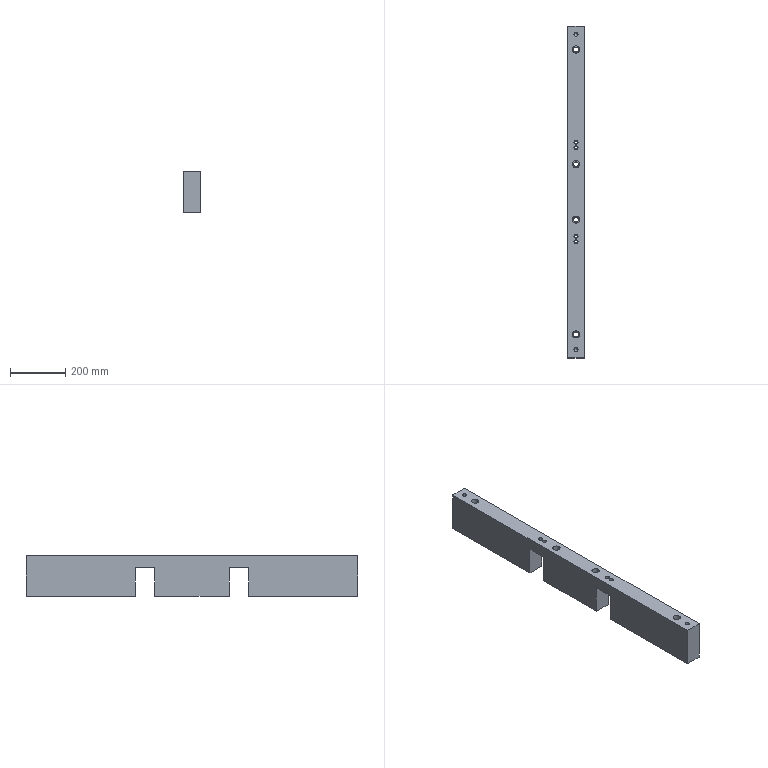Part | STEP file | lll_id2306_x_t | 1 solid | 42 faces | box 60 x 1200 x 147.5 mm | volume 9489564 mm3 | plane 22 | cylinder 18 | cone 2 | commonest cylinder face diameters 9.009 x4 14.508 x4 18.009 x4 26.008 x4 14.506 x2
STEP:
#1=CARTESIAN_POINT('',(1904.254,-179.998,370.));
#2=VERTEX_POINT('',#1);
#3=CARTESIAN_POINT('',(1897.,-179.998,370.));
#4=DIRECTION('',(0.,0.,-1.));
#5=DIRECTION('',(1.,0.,0.));
#6=AXIS2_PLACEMENT_3D('',#3,#4,#5);
#7=CIRCLE('',#6,7.254);
#8=EDGE_CURVE('',#2,#2,#7,.T.);
#9=ORIENTED_EDGE('',*,*,#8,.T.);
#10=EDGE_LOOP('',(#9));
#11=FACE_BOUND('',#10,.T.);
#12=CARTESIAN_POINT('',(1904.254,-159.998,370.));
#13=VERTEX_POINT('',#12);
#14=CARTESIAN_POINT('',(1897.,-159.998,370.));
#15=DIRECTION('',(0.,0.,-1.));
#16=DIRECTION('',(1.,0.,0.));
#17=AXIS2_PLACEMENT_3D('',#14,#15,#16);
#18=CIRCLE('',#17,7.254);
#19=EDGE_CURVE('',#13,#13,#18,.T.);
#20=ORIENTED_EDGE('',*,*,#19,.T.);
#21=EDGE_LOOP('',(#20));
#22=FACE_BOUND('',#21,.T.);
#23=CARTESIAN_POINT('',(1904.254,160.,370.));
#24=VERTEX_POINT('',#23);
#25=CARTESIAN_POINT('',(1897.,160.,370.));
#26=DIRECTION('',(0.,0.,-1.));
#27=DIRECTION('',(1.,0.,0.));
#28=AXIS2_PLACEMENT_3D('',#25,#26,#27);
#29=CIRCLE('',#28,7.254);
#30=EDGE_CURVE('',#24,#24,#29,.T.);
#31=ORIENTED_EDGE('',*,*,#30,.T.);
#32=EDGE_LOOP('',(#31));
#33=FACE_BOUND('',#32,.T.);
#34=CARTESIAN_POINT('',(1904.254,180.,370.));
#35=VERTEX_POINT('',#34);
#36=CARTESIAN_POINT('',(1897.,180.,370.));
#37=DIRECTION('',(0.,0.,-1.));
#38=DIRECTION('',(1.,0.,0.));
#39=AXIS2_PLACEMENT_3D('',#36,#37,#38);
#40=CIRCLE('',#39,7.254);
#41=EDGE_CURVE('',#35,#35,#40,.T.);
#42=ORIENTED_EDGE('',*,*,#41,.T.);
#43=EDGE_LOOP('',(#42));
#44=FACE_BOUND('',#43,.T.);
#45=CARTESIAN_POINT('',(1910.004,100.,370.));
#46=VERTEX_POINT('',#45);
#47=CARTESIAN_POINT('',(1897.,100.,370.));
#48=DIRECTION('',(0.,0.,1.));
#49=DIRECTION('',(1.,0.,0.));
#50=AXIS2_PLACEMENT_3D('',#47,#48,#49);
#51=CIRCLE('',#50,13.004);
#52=EDGE_CURVE('',#46,#46,#51,.T.);
#53=ORIENTED_EDGE('',*,*,#52,.F.);
#54=EDGE_LOOP('',(#53));
#55=FACE_BOUND('',#54,.T.);
#56=CARTESIAN_POINT('',(1910.004,-100.,370.));
#57=VERTEX_POINT('',#56);
#58=CARTESIAN_POINT('',(1897.,-100.,370.));
#59=DIRECTION('',(0.,0.,-1.));
#60=DIRECTION('',(1.,0.,0.));
#61=AXIS2_PLACEMENT_3D('',#58,#59,#60);
#62=CIRCLE('',#61,13.004);
#63=EDGE_CURVE('',#57,#57,#62,.T.);
#64=ORIENTED_EDGE('',*,*,#63,.T.);
#65=EDGE_LOOP('',(#64));
#66=FACE_BOUND('',#65,.T.);
#67=CARTESIAN_POINT('',(1910.004,-515.,370.));
#68=VERTEX_POINT('',#67);
#69=CARTESIAN_POINT('',(1897.,-515.,370.));
#70=DIRECTION('',(0.,0.,-1.));
#71=DIRECTION('',(1.,0.,0.));
#72=AXIS2_PLACEMENT_3D('',#69,#70,#71);
#73=CIRCLE('',#72,13.004);
#74=EDGE_CURVE('',#68,#68,#73,.T.);
#75=ORIENTED_EDGE('',*,*,#74,.T.);
#76=EDGE_LOOP('',(#75));
#77=FACE_BOUND('',#76,.T.);
#78=CARTESIAN_POINT('',(1927.,600.,370.));
#79=VERTEX_POINT('',#78);
#80=CARTESIAN_POINT('',(1867.,600.,370.));
#81=VERTEX_POINT('',#80);
#82=CARTESIAN_POINT('',(5837.,600.,370.));
#83=DIRECTION('',(-1.,0.,0.));
#84=VECTOR('',#83,1.);
#85=LINE('',#82,#84);
#86=EDGE_CURVE('',#79,#81,#85,.T.);
#87=ORIENTED_EDGE('',*,*,#86,.T.);
#88=CARTESIAN_POINT('',(1867.,-600.,370.));
#89=VERTEX_POINT('',#88);
#90=CARTESIAN_POINT('',(1867.,600.,370.));
#91=DIRECTION('',(0.,-1.,0.));
#92=VECTOR('',#91,1.);
#93=LINE('',#90,#92);
#94=EDGE_CURVE('',#81,#89,#93,.T.);
#95=ORIENTED_EDGE('',*,*,#94,.T.);
#96=CARTESIAN_POINT('',(1927.,-600.,370.));
#97=VERTEX_POINT('',#96);
#98=CARTESIAN_POINT('',(1867.,-600.,370.));
#99=DIRECTION('',(1.,0.,0.));
#100=VECTOR('',#99,1.);
#101=LINE('',#98,#100);
#102=EDGE_CURVE('',#89,#97,#101,.T.);
#103=ORIENTED_EDGE('',*,*,#102,.T.);
#104=CARTESIAN_POINT('',(1927.,1.,370.));
#105=DIRECTION('',(0.,1.,0.));
#106=VECTOR('',#105,1.);
#107=LINE('',#104,#106);
#108=EDGE_CURVE('',#97,#79,#107,.T.);
#109=ORIENTED_EDGE('',*,*,#108,.T.);
#110=EDGE_LOOP('',(#87,#95,#103,#109));
#111=FACE_BOUND('',#110,.T.);
#112=CARTESIAN_POINT('',(1910.004,515.,370.));
#113=VERTEX_POINT('',#112);
#114=CARTESIAN_POINT('',(1897.,515.,370.));
#115=DIRECTION('',(0.,0.,1.));
#116=DIRECTION('',(1.,0.,0.));
#117=AXIS2_PLACEMENT_3D('',#114,#115,#116);
#118=CIRCLE('',#117,13.004);
#119=EDGE_CURVE('',#113,#113,#118,.T.);
#120=ORIENTED_EDGE('',*,*,#119,.F.);
#121=EDGE_LOOP('',(#120));
#122=FACE_BOUND('',#121,.T.);
#123=CARTESIAN_POINT('',(1904.253,-570.,370.));
#124=VERTEX_POINT('',#123);
#125=CARTESIAN_POINT('',(1897.,-570.,370.));
#126=DIRECTION('',(0.,0.,-1.));
#127=DIRECTION('',(1.,0.,0.));
#128=AXIS2_PLACEMENT_3D('',#125,#126,#127);
#129=CIRCLE('',#128,7.253);
#130=EDGE_CURVE('',#124,#124,#129,.T.);
#131=ORIENTED_EDGE('',*,*,#130,.T.);
#132=EDGE_LOOP('',(#131));
#133=FACE_BOUND('',#132,.T.);
#134=CARTESIAN_POINT('',(1904.253,570.,370.));
#135=VERTEX_POINT('',#134);
#136=CARTESIAN_POINT('',(1897.,570.,370.));
#137=DIRECTION('',(0.,0.,1.));
#138=DIRECTION('',(1.,0.,0.));
#139=AXIS2_PLACEMENT_3D('',#136,#137,#138);
#140=CIRCLE('',#139,7.253);
#141=EDGE_CURVE('',#135,#135,#140,.T.);
#142=ORIENTED_EDGE('',*,*,#141,.F.);
#143=EDGE_LOOP('',(#142));
#144=FACE_BOUND('',#143,.T.);
#145=CARTESIAN_POINT('',(-319.315,1.,370.));
#146=DIRECTION('',(0.,0.,-1.));
#147=DIRECTION('',(1.,0.,0.));
#148=AXIS2_PLACEMENT_3D('',#145,#146,#147);
#149=PLANE('',#148);
#150=ADVANCED_FACE('',(#11,#22,#33,#44,#55,#66,#77,#111,#122,#133,#144),#149,.F.);
#151=CARTESIAN_POINT('',(1887.995,-100.,222.5));
#152=VERTEX_POINT('',#151);
#153=CARTESIAN_POINT('',(1897.,-100.,222.5));
#154=DIRECTION('',(0.,0.,1.));
#155=DIRECTION('',(-1.,0.,0.));
#156=AXIS2_PLACEMENT_3D('',#153,#154,#155);
#157=CIRCLE('',#156,9.005);
#158=EDGE_CURVE('',#152,#152,#157,.T.);
#159=ORIENTED_EDGE('',*,*,#158,.T.);
#160=EDGE_LOOP('',(#159));
#161=FACE_BOUND('',#160,.T.);
#162=CARTESIAN_POINT('',(1887.995,100.,222.5));
#163=VERTEX_POINT('',#162);
#164=CARTESIAN_POINT('',(1897.,100.,222.5));
#165=DIRECTION('',(0.,0.,-1.));
#166=DIRECTION('',(-1.,0.,0.));
#167=AXIS2_PLACEMENT_3D('',#164,#165,#166);
#168=CIRCLE('',#167,9.005);
#169=EDGE_CURVE('',#163,#163,#168,.T.);
#170=ORIENTED_EDGE('',*,*,#169,.F.);
#171=EDGE_LOOP('',(#170));
#172=FACE_BOUND('',#171,.T.);
#173=CARTESIAN_POINT('',(1927.,135.249,222.5));
#174=VERTEX_POINT('',#173);
#175=CARTESIAN_POINT('',(1867.,135.249,222.5));
#176=VERTEX_POINT('',#175);
#177=CARTESIAN_POINT('',(-319.315,135.249,222.5));
#178=DIRECTION('',(-1.,0.,0.));
#179=VECTOR('',#178,1.);
#180=LINE('',#177,#179);
#181=EDGE_CURVE('',#174,#176,#180,.T.);
#182=ORIENTED_EDGE('',*,*,#181,.F.);
#183=CARTESIAN_POINT('',(1927.,-134.749,222.5));
#184=VERTEX_POINT('',#183);
#185=CARTESIAN_POINT('',(1927.,1.,222.5));
#186=DIRECTION('',(0.,-1.,0.));
#187=VECTOR('',#186,1.);
#188=LINE('',#185,#187);
#189=EDGE_CURVE('',#174,#184,#188,.T.);
#190=ORIENTED_EDGE('',*,*,#189,.T.);
#191=CARTESIAN_POINT('',(1867.,-134.749,222.5));
#192=VERTEX_POINT('',#191);
#193=CARTESIAN_POINT('',(-319.315,-134.749,222.5));
#194=DIRECTION('',(1.,0.,0.));
#195=VECTOR('',#194,1.);
#196=LINE('',#193,#195);
#197=EDGE_CURVE('',#192,#184,#196,.T.);
#198=ORIENTED_EDGE('',*,*,#197,.F.);
#199=CARTESIAN_POINT('',(1867.,600.,222.5));
#200=DIRECTION('',(0.,-1.,0.));
#201=VECTOR('',#200,1.);
#202=LINE('',#199,#201);
#203=EDGE_CURVE('',#176,#192,#202,.T.);
#204=ORIENTED_EDGE('',*,*,#203,.F.);
#205=EDGE_LOOP('',(#182,#190,#198,#204));
#206=FACE_BOUND('',#205,.T.);
#207=CARTESIAN_POINT('',(-319.315,1.,222.5));
#208=DIRECTION('',(0.,0.,-1.));
#209=DIRECTION('',(1.,0.,0.));
#210=AXIS2_PLACEMENT_3D('',#207,#208,#209);
#211=PLANE('',#210);
#212=ADVANCED_FACE('',(#161,#172,#206),#211,.T.);
#213=CARTESIAN_POINT('',(1867.,205.249,222.5));
#214=VERTEX_POINT('',#213);
#215=CARTESIAN_POINT('',(1927.,205.249,222.5));
#216=VERTEX_POINT('',#215);
#217=CARTESIAN_POINT('',(-319.315,205.249,222.5));
#218=DIRECTION('',(1.,0.,0.));
#219=VECTOR('',#218,1.);
#220=LINE('',#217,#219);
#221=EDGE_CURVE('',#214,#216,#220,.T.);
#222=ORIENTED_EDGE('',*,*,#221,.F.);
#223=CARTESIAN_POINT('',(1867.,600.,222.5));
#224=VERTEX_POINT('',#223);
#225=CARTESIAN_POINT('',(1867.,600.,222.5));
#226=DIRECTION('',(0.,-1.,0.));
#227=VECTOR('',#226,1.);
#228=LINE('',#225,#227);
#229=EDGE_CURVE('',#224,#214,#228,.T.);
#230=ORIENTED_EDGE('',*,*,#229,.F.);
#231=CARTESIAN_POINT('',(1927.,600.,222.5));
#232=VERTEX_POINT('',#231);
#233=CARTESIAN_POINT('',(5837.,600.,222.5));
#234=DIRECTION('',(-1.,0.,0.));
#235=VECTOR('',#234,1.);
#236=LINE('',#233,#235);
#237=EDGE_CURVE('',#232,#224,#236,.T.);
#238=ORIENTED_EDGE('',*,*,#237,.F.);
#239=CARTESIAN_POINT('',(1927.,1.,222.5));
#240=DIRECTION('',(0.,-1.,0.));
#241=VECTOR('',#240,1.);
#242=LINE('',#239,#241);
#243=EDGE_CURVE('',#232,#216,#242,.T.);
#244=ORIENTED_EDGE('',*,*,#243,.T.);
#245=EDGE_LOOP('',(#222,#230,#238,#244));
#246=FACE_BOUND('',#245,.T.);
#247=CARTESIAN_POINT('',(1906.005,515.,222.5));
#248=VERTEX_POINT('',#247);
#249=CARTESIAN_POINT('',(1897.,515.,222.5));
#250=DIRECTION('',(0.,0.,-1.));
#251=DIRECTION('',(1.,0.,0.));
#252=AXIS2_PLACEMENT_3D('',#249,#250,#251);
#253=CIRCLE('',#252,9.005);
#254=EDGE_CURVE('',#248,#248,#253,.T.);
#255=ORIENTED_EDGE('',*,*,#254,.F.);
#256=EDGE_LOOP('',(#255));
#257=FACE_BOUND('',#256,.T.);
#258=CARTESIAN_POINT('',(-319.315,1.,222.5));
#259=DIRECTION('',(0.,0.,-1.));
#260=DIRECTION('',(1.,0.,0.));
#261=AXIS2_PLACEMENT_3D('',#258,#259,#260);
#262=PLANE('',#261);
#263=ADVANCED_FACE('',(#246,#257),#262,.T.);
#264=CARTESIAN_POINT('',(1927.,-204.749,222.5));
#265=VERTEX_POINT('',#264);
#266=CARTESIAN_POINT('',(1867.,-204.749,222.5));
#267=VERTEX_POINT('',#266);
#268=CARTESIAN_POINT('',(-319.315,-204.749,222.5));
#269=DIRECTION('',(-1.,0.,0.));
#270=VECTOR('',#269,1.);
#271=LINE('',#268,#270);
#272=EDGE_CURVE('',#265,#267,#271,.T.);
#273=ORIENTED_EDGE('',*,*,#272,.F.);
#274=CARTESIAN_POINT('',(1927.,-600.,222.5));
#275=VERTEX_POINT('',#274);
#276=CARTESIAN_POINT('',(1927.,1.,222.5));
#277=DIRECTION('',(0.,-1.,0.));
#278=VECTOR('',#277,1.);
#279=LINE('',#276,#278);
#280=EDGE_CURVE('',#265,#275,#279,.T.);
#281=ORIENTED_EDGE('',*,*,#280,.T.);
#282=CARTESIAN_POINT('',(1867.,-600.,222.5));
#283=VERTEX_POINT('',#282);
#284=CARTESIAN_POINT('',(1867.,-600.,222.5));
#285=DIRECTION('',(1.,0.,0.));
#286=VECTOR('',#285,1.);
#287=LINE('',#284,#286);
#288=EDGE_CURVE('',#283,#275,#287,.T.);
#289=ORIENTED_EDGE('',*,*,#288,.F.);
#290=CARTESIAN_POINT('',(1867.,600.,222.5));
#291=DIRECTION('',(0.,-1.,0.));
#292=VECTOR('',#291,1.);
#293=LINE('',#290,#292);
#294=EDGE_CURVE('',#267,#283,#293,.T.);
#295=ORIENTED_EDGE('',*,*,#294,.F.);
#296=EDGE_LOOP('',(#273,#281,#289,#295));
#297=FACE_BOUND('',#296,.T.);
#298=CARTESIAN_POINT('',(1906.005,-515.,222.5));
#299=VERTEX_POINT('',#298);
#300=CARTESIAN_POINT('',(1897.,-515.,222.5));
#301=DIRECTION('',(0.,0.,1.));
#302=DIRECTION('',(1.,0.,0.));
#303=AXIS2_PLACEMENT_3D('',#300,#301,#302);
#304=CIRCLE('',#303,9.005);
#305=EDGE_CURVE('',#299,#299,#304,.T.);
#306=ORIENTED_EDGE('',*,*,#305,.T.);
#307=EDGE_LOOP('',(#306));
#308=FACE_BOUND('',#307,.T.);
#309=CARTESIAN_POINT('',(-319.315,1.,222.5));
#310=DIRECTION('',(0.,0.,-1.));
#311=DIRECTION('',(1.,0.,0.));
#312=AXIS2_PLACEMENT_3D('',#309,#310,#311);
#313=PLANE('',#312);
#314=ADVANCED_FACE('',(#297,#308),#313,.T.);
#315=CARTESIAN_POINT('',(1867.,-134.749,326.5));
#316=VERTEX_POINT('',#315);
#317=CARTESIAN_POINT('',(1867.,-204.749,326.5));
#318=VERTEX_POINT('',#317);
#319=CARTESIAN_POINT('',(1867.,80.002,326.5));
#320=DIRECTION('',(0.,-1.,0.));
#321=VECTOR('',#320,1.);
#322=LINE('',#319,#321);
#323=EDGE_CURVE('',#316,#318,#322,.T.);
#324=ORIENTED_EDGE('',*,*,#323,.T.);
#325=CARTESIAN_POINT('',(1867.,-204.749,363.5));
#326=DIRECTION('',(0.,0.,1.));
#327=VECTOR('',#326,1.);
#328=LINE('',#325,#327);
#329=EDGE_CURVE('',#267,#318,#328,.T.);
#330=ORIENTED_EDGE('',*,*,#329,.F.);
#331=ORIENTED_EDGE('',*,*,#294,.T.);
#332=CARTESIAN_POINT('',(1867.,-600.,310.));
#333=DIRECTION('',(0.,0.,-1.));
#334=VECTOR('',#333,1.);
#335=LINE('',#332,#334);
#336=EDGE_CURVE('',#89,#283,#335,.T.);
#337=ORIENTED_EDGE('',*,*,#336,.F.);
#338=ORIENTED_EDGE('',*,*,#94,.F.);
#339=CARTESIAN_POINT('',(1867.,600.,310.));
#340=DIRECTION('',(0.,0.,-1.));
#341=VECTOR('',#340,1.);
#342=LINE('',#339,#341);
#343=EDGE_CURVE('',#81,#224,#342,.T.);
#344=ORIENTED_EDGE('',*,*,#343,.T.);
#345=ORIENTED_EDGE('',*,*,#229,.T.);
#346=CARTESIAN_POINT('',(1867.,205.249,326.5));
#347=VERTEX_POINT('',#346);
#348=CARTESIAN_POINT('',(1867.,205.249,363.5));
#349=DIRECTION('',(0.,0.,-1.));
#350=VECTOR('',#349,1.);
#351=LINE('',#348,#350);
#352=EDGE_CURVE('',#347,#214,#351,.T.);
#353=ORIENTED_EDGE('',*,*,#352,.F.);
#354=CARTESIAN_POINT('',(1867.,135.249,326.5));
#355=VERTEX_POINT('',#354);
#356=CARTESIAN_POINT('',(1867.,420.,326.5));
#357=DIRECTION('',(0.,-1.,0.));
#358=VECTOR('',#357,1.);
#359=LINE('',#356,#358);
#360=EDGE_CURVE('',#347,#355,#359,.T.);
#361=ORIENTED_EDGE('',*,*,#360,.T.);
#362=CARTESIAN_POINT('',(1867.,135.249,363.5));
#363=DIRECTION('',(0.,0.,1.));
#364=VECTOR('',#363,1.);
#365=LINE('',#362,#364);
#366=EDGE_CURVE('',#176,#355,#365,.T.);
#367=ORIENTED_EDGE('',*,*,#366,.F.);
#368=ORIENTED_EDGE('',*,*,#203,.T.);
#369=CARTESIAN_POINT('',(1867.,-134.749,363.5));
#370=DIRECTION('',(0.,0.,-1.));
#371=VECTOR('',#370,1.);
#372=LINE('',#369,#371);
#373=EDGE_CURVE('',#316,#192,#372,.T.);
#374=ORIENTED_EDGE('',*,*,#373,.F.);
#375=EDGE_LOOP('',(#324,#330,#331,#337,#338,#344,#345,#353,#361,#367,#368,#374));
#376=FACE_OUTER_BOUND('',#375,.T.);
#377=CARTESIAN_POINT('',(1867.,600.,310.));
#378=DIRECTION('',(-1.,0.,0.));
#379=DIRECTION('',(0.,0.,-1.));
#380=AXIS2_PLACEMENT_3D('',#377,#378,#379);
#381=PLANE('',#380);
#382=ADVANCED_FACE('',(#376),#381,.T.);
#383=CARTESIAN_POINT('',(1927.,-600.,310.));
#384=DIRECTION('',(0.,0.,-1.));
#385=VECTOR('',#384,1.);
#386=LINE('',#383,#385);
#387=EDGE_CURVE('',#97,#275,#386,.T.);
#388=ORIENTED_EDGE('',*,*,#387,.F.);
#389=ORIENTED_EDGE('',*,*,#102,.F.);
#390=ORIENTED_EDGE('',*,*,#336,.T.);
#391=ORIENTED_EDGE('',*,*,#288,.T.);
#392=EDGE_LOOP('',(#388,#389,#390,#391));
#393=FACE_OUTER_BOUND('',#392,.T.);
#394=CARTESIAN_POINT('',(1867.,-600.,310.));
#395=DIRECTION('',(0.,-1.,0.));
#396=DIRECTION('',(0.,0.,-1.));
#397=AXIS2_PLACEMENT_3D('',#394,#395,#396);
#398=PLANE('',#397);
#399=ADVANCED_FACE('',(#393),#398,.T.);
#400=CARTESIAN_POINT('',(1927.,600.,310.));
#401=DIRECTION('',(0.,0.,1.));
#402=VECTOR('',#401,1.);
#403=LINE('',#400,#402);
#404=EDGE_CURVE('',#232,#79,#403,.T.);
#405=ORIENTED_EDGE('',*,*,#404,.F.);
#406=ORIENTED_EDGE('',*,*,#237,.T.);
#407=ORIENTED_EDGE('',*,*,#343,.F.);
#408=ORIENTED_EDGE('',*,*,#86,.F.);
#409=EDGE_LOOP('',(#405,#406,#407,#408));
#410=FACE_OUTER_BOUND('',#409,.T.);
#411=CARTESIAN_POINT('',(5837.,600.,310.));
#412=DIRECTION('',(0.,1.,0.));
#413=DIRECTION('',(0.,0.,1.));
#414=AXIS2_PLACEMENT_3D('',#411,#412,#413);
#415=PLANE('',#414);
#416=ADVANCED_FACE('',(#410),#415,.T.);
#417=CARTESIAN_POINT('',(1927.,-204.749,326.5));
#418=VERTEX_POINT('',#417);
#419=CARTESIAN_POINT('',(1927.,-204.749,294.75));
#420=DIRECTION('',(0.,0.,1.));
#421=VECTOR('',#420,1.);
#422=LINE('',#419,#421);
#423=EDGE_CURVE('',#265,#418,#422,.T.);
#424=ORIENTED_EDGE('',*,*,#423,.T.);
#425=CARTESIAN_POINT('',(1927.,-134.749,326.5));
#426=VERTEX_POINT('',#425);
#427=CARTESIAN_POINT('',(1927.,-519.998,326.5));
#428=DIRECTION('',(0.,-1.,0.));
#429=VECTOR('',#428,1.);
#430=LINE('',#427,#429);
#431=EDGE_CURVE('',#426,#418,#430,.T.);
#432=ORIENTED_EDGE('',*,*,#431,.F.);
#433=CARTESIAN_POINT('',(1927.,-134.749,294.75));
#434=DIRECTION('',(0.,0.,-1.));
#435=VECTOR('',#434,1.);
#436=LINE('',#433,#435);
#437=EDGE_CURVE('',#426,#184,#436,.T.);
#438=ORIENTED_EDGE('',*,*,#437,.T.);
#439=ORIENTED_EDGE('',*,*,#189,.F.);
#440=CARTESIAN_POINT('',(1927.,135.249,326.5));
#441=VERTEX_POINT('',#440);
#442=CARTESIAN_POINT('',(1927.,135.249,294.75));
#443=DIRECTION('',(0.,0.,1.));
#444=VECTOR('',#443,1.);
#445=LINE('',#442,#444);
#446=EDGE_CURVE('',#174,#441,#445,.T.);
#447=ORIENTED_EDGE('',*,*,#446,.T.);
#448=CARTESIAN_POINT('',(1927.,205.249,326.5));
#449=VERTEX_POINT('',#448);
#450=CARTESIAN_POINT('',(1927.,-180.,326.5));
#451=DIRECTION('',(0.,-1.,0.));
#452=VECTOR('',#451,1.);
#453=LINE('',#450,#452);
#454=EDGE_CURVE('',#449,#441,#453,.T.);
#455=ORIENTED_EDGE('',*,*,#454,.F.);
#456=CARTESIAN_POINT('',(1927.,205.249,294.75));
#457=DIRECTION('',(0.,0.,-1.));
#458=VECTOR('',#457,1.);
#459=LINE('',#456,#458);
#460=EDGE_CURVE('',#449,#216,#459,.T.);
#461=ORIENTED_EDGE('',*,*,#460,.T.);
#462=ORIENTED_EDGE('',*,*,#243,.F.);
#463=ORIENTED_EDGE('',*,*,#404,.T.);
#464=ORIENTED_EDGE('',*,*,#108,.F.);
#465=ORIENTED_EDGE('',*,*,#387,.T.);
#466=ORIENTED_EDGE('',*,*,#280,.F.);
#467=EDGE_LOOP('',(#424,#432,#438,#439,#447,#455,#461,#462,#463,#464,#465,#466));
#468=FACE_OUTER_BOUND('',#467,.T.);
#469=CARTESIAN_POINT('',(1927.,0.,241.25));
#470=DIRECTION('',(-1.,0.,0.));
#471=DIRECTION('',(0.,0.,-1.));
#472=AXIS2_PLACEMENT_3D('',#469,#470,#471);
#473=PLANE('',#472);
#474=ADVANCED_FACE('',(#468),#473,.F.);
#475=CARTESIAN_POINT('',(1887.995,-515.,302.5));
#476=VERTEX_POINT('',#475);
#477=CARTESIAN_POINT('',(1897.,-515.,302.5));
#478=DIRECTION('',(0.,0.,-1.));
#479=DIRECTION('',(-1.,0.,0.));
#480=AXIS2_PLACEMENT_3D('',#477,#478,#479);
#481=CIRCLE('',#480,9.005);
#482=EDGE_CURVE('',#476,#476,#481,.T.);
#483=ORIENTED_EDGE('',*,*,#482,.F.);
#484=EDGE_LOOP('',(#483));
#485=FACE_BOUND('',#484,.T.);
#486=ORIENTED_EDGE('',*,*,#305,.F.);
#487=EDGE_LOOP('',(#486));
#488=FACE_BOUND('',#487,.T.);
#489=CARTESIAN_POINT('',(1897.,-515.,420.));
#490=DIRECTION('',(0.,0.,-1.));
#491=DIRECTION('',(1.,0.,0.));
#492=AXIS2_PLACEMENT_3D('',#489,#490,#491);
#493=CYLINDRICAL_SURFACE('',#492,9.005);
#494=ADVANCED_FACE('',(#485,#488),#493,.F.);
#495=ORIENTED_EDGE('',*,*,#482,.T.);
#496=EDGE_LOOP('',(#495));
#497=FACE_BOUND('',#496,.T.);
#498=CARTESIAN_POINT('',(1910.004,-515.,302.5));
#499=VERTEX_POINT('',#498);
#500=CARTESIAN_POINT('',(1897.,-515.,302.5));
#501=DIRECTION('',(0.,0.,-1.));
#502=DIRECTION('',(-1.,0.,0.));
#503=AXIS2_PLACEMENT_3D('',#500,#501,#502);
#504=CIRCLE('',#503,13.004);
#505=EDGE_CURVE('',#499,#499,#504,.T.);
#506=ORIENTED_EDGE('',*,*,#505,.F.);
#507=EDGE_LOOP('',(#506));
#508=FACE_BOUND('',#507,.T.);
#509=CARTESIAN_POINT('',(1897.,-515.,302.5));
#510=DIRECTION('',(0.,0.,-1.));
#511=DIRECTION('',(-1.,0.,0.));
#512=AXIS2_PLACEMENT_3D('',#509,#510,#511);
#513=PLANE('',#512);
#514=ADVANCED_FACE('',(#497,#508),#513,.F.);
#515=ORIENTED_EDGE('',*,*,#505,.T.);
#516=EDGE_LOOP('',(#515));
#517=FACE_BOUND('',#516,.T.);
#518=ORIENTED_EDGE('',*,*,#74,.F.);
#519=EDGE_LOOP('',(#518));
#520=FACE_BOUND('',#519,.T.);
#521=CARTESIAN_POINT('',(1897.,-515.,370.));
#522=DIRECTION('',(0.,0.,-1.));
#523=DIRECTION('',(1.,0.,0.));
#524=AXIS2_PLACEMENT_3D('',#521,#522,#523);
#525=CYLINDRICAL_SURFACE('',#524,13.004);
#526=ADVANCED_FACE('',(#517,#520),#525,.F.);
#527=CARTESIAN_POINT('',(1887.995,-100.,302.5));
#528=VERTEX_POINT('',#527);
#529=CARTESIAN_POINT('',(1897.,-100.,302.5));
#530=DIRECTION('',(0.,0.,-1.));
#531=DIRECTION('',(-1.,0.,0.));
#532=AXIS2_PLACEMENT_3D('',#529,#530,#531);
#533=CIRCLE('',#532,9.005);
#534=EDGE_CURVE('',#528,#528,#533,.T.);
#535=ORIENTED_EDGE('',*,*,#534,.F.);
#536=EDGE_LOOP('',(#535));
#537=FACE_BOUND('',#536,.T.);
#538=ORIENTED_EDGE('',*,*,#158,.F.);
#539=EDGE_LOOP('',(#538));
#540=FACE_BOUND('',#539,.T.);
#541=CARTESIAN_POINT('',(1897.,-100.,420.));
#542=DIRECTION('',(0.,0.,-1.));
#543=DIRECTION('',(1.,0.,0.));
#544=AXIS2_PLACEMENT_3D('',#541,#542,#543);
#545=CYLINDRICAL_SURFACE('',#544,9.005);
#546=ADVANCED_FACE('',(#537,#540),#545,.F.);
#547=ORIENTED_EDGE('',*,*,#534,.T.);
#548=EDGE_LOOP('',(#547));
#549=FACE_BOUND('',#548,.T.);
#550=CARTESIAN_POINT('',(1910.004,-100.,302.5));
#551=VERTEX_POINT('',#550);
#552=CARTESIAN_POINT('',(1897.,-100.,302.5));
#553=DIRECTION('',(0.,0.,-1.));
#554=DIRECTION('',(1.,0.,0.));
#555=AXIS2_PLACEMENT_3D('',#552,#553,#554);
#556=CIRCLE('',#555,13.004);
#557=EDGE_CURVE('',#551,#551,#556,.T.);
#558=ORIENTED_EDGE('',*,*,#557,.F.);
#559=EDGE_LOOP('',(#558));
#560=FACE_BOUND('',#559,.T.);
#561=CARTESIAN_POINT('',(1897.,-100.,302.5));
#562=DIRECTION('',(0.,0.,-1.));
#563=DIRECTION('',(-1.,0.,0.));
#564=AXIS2_PLACEMENT_3D('',#561,#562,#563);
#565=PLANE('',#564);
#566=ADVANCED_FACE('',(#549,#560),#565,.F.);
#567=ORIENTED_EDGE('',*,*,#557,.T.);
#568=EDGE_LOOP('',(#567));
#569=FACE_BOUND('',#568,.T.);
#570=ORIENTED_EDGE('',*,*,#63,.F.);
#571=EDGE_LOOP('',(#570));
#572=FACE_BOUND('',#571,.T.);
#573=CARTESIAN_POINT('',(1897.,-100.,370.));
#574=DIRECTION('',(0.,0.,-1.));
#575=DIRECTION('',(1.,0.,0.));
#576=AXIS2_PLACEMENT_3D('',#573,#574,#575);
#577=CYLINDRICAL_SURFACE('',#576,13.004);
#578=ADVANCED_FACE('',(#569,#572),#577,.F.);
#579=CARTESIAN_POINT('',(1887.995,100.,302.5));
#580=VERTEX_POINT('',#579);
#581=CARTESIAN_POINT('',(1897.,100.,302.5));
#582=DIRECTION('',(0.,0.,1.));
#583=DIRECTION('',(-1.,0.,0.));
#584=AXIS2_PLACEMENT_3D('',#581,#582,#583);
#585=CIRCLE('',#584,9.005);
#586=EDGE_CURVE('',#580,#580,#585,.T.);
#587=ORIENTED_EDGE('',*,*,#586,.T.);
#588=EDGE_LOOP('',(#587));
#589=FACE_BOUND('',#588,.T.);
#590=ORIENTED_EDGE('',*,*,#169,.T.);
#591=EDGE_LOOP('',(#590));
#592=FACE_BOUND('',#591,.T.);
#593=CARTESIAN_POINT('',(1897.,100.,420.));
#594=DIRECTION('',(0.,0.,-1.));
#595=DIRECTION('',(1.,0.,0.));
#596=AXIS2_PLACEMENT_3D('',#593,#594,#595);
#597=CYLINDRICAL_SURFACE('',#596,9.005);
#598=ADVANCED_FACE('',(#589,#592),#597,.F.);
#599=ORIENTED_EDGE('',*,*,#586,.F.);
#600=EDGE_LOOP('',(#599));
#601=FACE_BOUND('',#600,.T.);
#602=CARTESIAN_POINT('',(1910.004,100.,302.5));
#603=VERTEX_POINT('',#602);
#604=CARTESIAN_POINT('',(1897.,100.,302.5));
#605=DIRECTION('',(0.,0.,1.));
#606=DIRECTION('',(1.,0.,0.));
#607=AXIS2_PLACEMENT_3D('',#604,#605,#606);
#608=CIRCLE('',#607,13.004);
#609=EDGE_CURVE('',#603,#603,#608,.T.);
#610=ORIENTED_EDGE('',*,*,#609,.T.);
#611=EDGE_LOOP('',(#610));
#612=FACE_BOUND('',#611,.T.);
#613=CARTESIAN_POINT('',(1897.,100.,302.5));
#614=DIRECTION('',(0.,0.,-1.));
#615=DIRECTION('',(-1.,0.,0.));
#616=AXIS2_PLACEMENT_3D('',#613,#614,#615);
#617=PLANE('',#616);
#618=ADVANCED_FACE('',(#601,#612),#617,.F.);
#619=ORIENTED_EDGE('',*,*,#609,.F.);
#620=EDGE_LOOP('',(#619));
#621=FACE_BOUND('',#620,.T.);
#622=ORIENTED_EDGE('',*,*,#52,.T.);
#623=EDGE_LOOP('',(#622));
#624=FACE_BOUND('',#623,.T.);
#625=CARTESIAN_POINT('',(1897.,100.,370.));
#626=DIRECTION('',(0.,0.,-1.));
#627=DIRECTION('',(1.,0.,0.));
#628=AXIS2_PLACEMENT_3D('',#625,#626,#627);
#629=CYLINDRICAL_SURFACE('',#628,13.004);
#630=ADVANCED_FACE('',(#621,#624),#629,.F.);
#631=CARTESIAN_POINT('',(1887.995,515.,302.5));
#632=VERTEX_POINT('',#631);
#633=CARTESIAN_POINT('',(1897.,515.,302.5));
#634=DIRECTION('',(0.,0.,1.));
#635=DIRECTION('',(-1.,0.,0.));
#636=AXIS2_PLACEMENT_3D('',#633,#634,#635);
#637=CIRCLE('',#636,9.005);
#638=EDGE_CURVE('',#632,#632,#637,.T.);
#639=ORIENTED_EDGE('',*,*,#638,.T.);
#640=EDGE_LOOP('',(#639));
#641=FACE_BOUND('',#640,.T.);
#642=ORIENTED_EDGE('',*,*,#254,.T.);
#643=EDGE_LOOP('',(#642));
#644=FACE_BOUND('',#643,.T.);
#645=CARTESIAN_POINT('',(1897.,515.,420.));
#646=DIRECTION('',(0.,0.,-1.));
#647=DIRECTION('',(1.,0.,0.));
#648=AXIS2_PLACEMENT_3D('',#645,#646,#647);
#649=CYLINDRICAL_SURFACE('',#648,9.005);
#650=ADVANCED_FACE('',(#641,#644),#649,.F.);
#651=ORIENTED_EDGE('',*,*,#638,.F.);
#652=EDGE_LOOP('',(#651));
#653=FACE_BOUND('',#652,.T.);
#654=CARTESIAN_POINT('',(1910.004,515.,302.5));
#655=VERTEX_POINT('',#654);
#656=CARTESIAN_POINT('',(1897.,515.,302.5));
#657=DIRECTION('',(0.,0.,1.));
#658=DIRECTION('',(1.,0.,0.));
#659=AXIS2_PLACEMENT_3D('',#656,#657,#658);
#660=CIRCLE('',#659,13.004);
#661=EDGE_CURVE('',#655,#655,#660,.T.);
#662=ORIENTED_EDGE('',*,*,#661,.T.);
#663=EDGE_LOOP('',(#662));
#664=FACE_BOUND('',#663,.T.);
#665=CARTESIAN_POINT('',(1897.,515.,302.5));
#666=DIRECTION('',(0.,0.,-1.));
#667=DIRECTION('',(-1.,0.,0.));
#668=AXIS2_PLACEMENT_3D('',#665,#666,#667);
#669=PLANE('',#668);
#670=ADVANCED_FACE('',(#653,#664),#669,.F.);
#671=ORIENTED_EDGE('',*,*,#661,.F.);
#672=EDGE_LOOP('',(#671));
#673=FACE_BOUND('',#672,.T.);
#674=ORIENTED_EDGE('',*,*,#119,.T.);
#675=EDGE_LOOP('',(#674));
#676=FACE_BOUND('',#675,.T.);
#677=CARTESIAN_POINT('',(1897.,515.,370.));
#678=DIRECTION('',(0.,0.,-1.));
#679=DIRECTION('',(1.,0.,0.));
#680=AXIS2_PLACEMENT_3D('',#677,#678,#679);
#681=CYLINDRICAL_SURFACE('',#680,13.004);
#682=ADVANCED_FACE('',(#673,#676),#681,.F.);
#683=ORIENTED_EDGE('',*,*,#373,.T.);
#684=ORIENTED_EDGE('',*,*,#197,.T.);
#685=ORIENTED_EDGE('',*,*,#437,.F.);
#686=CARTESIAN_POINT('',(1897.,-134.749,326.5));
#687=DIRECTION('',(-1.,0.,0.));
#688=VECTOR('',#687,1.);
#689=LINE('',#686,#688);
#690=EDGE_CURVE('',#426,#316,#689,.T.);
#691=ORIENTED_EDGE('',*,*,#690,.T.);
#692=EDGE_LOOP('',(#683,#684,#685,#691));
#693=FACE_OUTER_BOUND('',#692,.T.);
#694=CARTESIAN_POINT('',(1897.,-134.749,130.));
#695=DIRECTION('',(0.,1.,0.));
#696=DIRECTION('',(0.,0.,-1.));
#697=AXIS2_PLACEMENT_3D('',#694,#695,#696);
#698=PLANE('',#697);
#699=ADVANCED_FACE('',(#693),#698,.F.);
#700=ORIENTED_EDGE('',*,*,#329,.T.);
#701=CARTESIAN_POINT('',(1897.,-204.749,326.5));
#702=DIRECTION('',(1.,0.,0.));
#703=VECTOR('',#702,1.);
#704=LINE('',#701,#703);
#705=EDGE_CURVE('',#318,#418,#704,.T.);
#706=ORIENTED_EDGE('',*,*,#705,.T.);
#707=ORIENTED_EDGE('',*,*,#423,.F.);
#708=ORIENTED_EDGE('',*,*,#272,.T.);
#709=EDGE_LOOP('',(#700,#706,#707,#708));
#710=FACE_OUTER_BOUND('',#709,.T.);
#711=CARTESIAN_POINT('',(1897.,-204.749,130.));
#712=DIRECTION('',(0.,-1.,0.));
#713=DIRECTION('',(0.,0.,1.));
#714=AXIS2_PLACEMENT_3D('',#711,#712,#713);
#715=PLANE('',#714);
#716=ADVANCED_FACE('',(#710),#715,.F.);
#717=ORIENTED_EDGE('',*,*,#366,.T.);
#718=CARTESIAN_POINT('',(1897.,135.249,326.5));
#719=DIRECTION('',(1.,0.,0.));
#720=VECTOR('',#719,1.);
#721=LINE('',#718,#720);
#722=EDGE_CURVE('',#355,#441,#721,.T.);
#723=ORIENTED_EDGE('',*,*,#722,.T.);
#724=ORIENTED_EDGE('',*,*,#446,.F.);
#725=ORIENTED_EDGE('',*,*,#181,.T.);
#726=EDGE_LOOP('',(#717,#723,#724,#725));
#727=FACE_OUTER_BOUND('',#726,.T.);
#728=CARTESIAN_POINT('',(1897.,135.249,130.));
#729=DIRECTION('',(0.,-1.,0.));
#730=DIRECTION('',(0.,0.,-1.));
#731=AXIS2_PLACEMENT_3D('',#728,#729,#730);
#732=PLANE('',#731);
#733=ADVANCED_FACE('',(#727),#732,.F.);
#734=ORIENTED_EDGE('',*,*,#352,.T.);
#735=ORIENTED_EDGE('',*,*,#221,.T.);
#736=ORIENTED_EDGE('',*,*,#460,.F.);
#737=CARTESIAN_POINT('',(1897.,205.249,326.5));
#738=DIRECTION('',(-1.,0.,0.));
#739=VECTOR('',#738,1.);
#740=LINE('',#737,#739);
#741=EDGE_CURVE('',#449,#347,#740,.T.);
#742=ORIENTED_EDGE('',*,*,#741,.T.);
#743=EDGE_LOOP('',(#734,#735,#736,#742));
#744=FACE_OUTER_BOUND('',#743,.T.);
#745=CARTESIAN_POINT('',(1897.,205.249,130.));
#746=DIRECTION('',(0.,1.,0.));
#747=DIRECTION('',(0.,0.,1.));
#748=AXIS2_PLACEMENT_3D('',#745,#746,#747);
#749=PLANE('',#748);
#750=ADVANCED_FACE('',(#744),#749,.F.);
#751=CARTESIAN_POINT('',(1904.254,160.,351.5));
#752=VERTEX_POINT('',#751);
#753=CARTESIAN_POINT('',(1897.,160.,351.5));
#754=DIRECTION('',(0.,0.,-1.));
#755=DIRECTION('',(1.,0.,0.));
#756=AXIS2_PLACEMENT_3D('',#753,#754,#755);
#757=CIRCLE('',#756,7.254);
#758=EDGE_CURVE('',#752,#752,#757,.T.);
#759=ORIENTED_EDGE('',*,*,#758,.T.);
#760=EDGE_LOOP('',(#759));
#761=FACE_BOUND('',#760,.T.);
#762=ORIENTED_EDGE('',*,*,#30,.F.);
#763=EDGE_LOOP('',(#762));
#764=FACE_BOUND('',#763,.T.);
#765=CARTESIAN_POINT('',(1897.,160.,370.));
#766=DIRECTION('',(0.,0.,-1.));
#767=DIRECTION('',(1.,0.,0.));
#768=AXIS2_PLACEMENT_3D('',#765,#766,#767);
#769=CYLINDRICAL_SURFACE('',#768,7.254);
#770=ADVANCED_FACE('',(#761,#764),#769,.F.);
#771=CARTESIAN_POINT('',(1904.254,180.,351.5));
#772=VERTEX_POINT('',#771);
#773=CARTESIAN_POINT('',(1897.,180.,351.5));
#774=DIRECTION('',(0.,0.,-1.));
#775=DIRECTION('',(1.,0.,0.));
#776=AXIS2_PLACEMENT_3D('',#773,#774,#775);
#777=CIRCLE('',#776,7.254);
#778=EDGE_CURVE('',#772,#772,#777,.T.);
#779=ORIENTED_EDGE('',*,*,#778,.T.);
#780=EDGE_LOOP('',(#779));
#781=FACE_BOUND('',#780,.T.);
#782=ORIENTED_EDGE('',*,*,#41,.F.);
#783=EDGE_LOOP('',(#782));
#784=FACE_BOUND('',#783,.T.);
#785=CARTESIAN_POINT('',(1897.,180.,370.));
#786=DIRECTION('',(0.,0.,-1.));
#787=DIRECTION('',(1.,0.,0.));
#788=AXIS2_PLACEMENT_3D('',#785,#786,#787);
#789=CYLINDRICAL_SURFACE('',#788,7.254);
#790=ADVANCED_FACE('',(#781,#784),#789,.F.);
#791=CARTESIAN_POINT('',(1892.495,180.,351.5));
#792=VERTEX_POINT('',#791);
#793=CARTESIAN_POINT('',(1897.,180.,351.5));
#794=DIRECTION('',(0.,0.,-1.));
#795=DIRECTION('',(-1.,0.,0.));
#796=AXIS2_PLACEMENT_3D('',#793,#794,#795);
#797=CIRCLE('',#796,4.505);
#798=EDGE_CURVE('',#792,#792,#797,.T.);
#799=ORIENTED_EDGE('',*,*,#798,.T.);
#800=EDGE_LOOP('',(#799));
#801=FACE_BOUND('',#800,.T.);
#802=ORIENTED_EDGE('',*,*,#778,.F.);
#803=EDGE_LOOP('',(#802));
#804=FACE_BOUND('',#803,.T.);
#805=CARTESIAN_POINT('',(1897.,180.,351.5));
#806=DIRECTION('',(0.,0.,-1.));
#807=DIRECTION('',(-1.,0.,0.));
#808=AXIS2_PLACEMENT_3D('',#805,#806,#807);
#809=PLANE('',#808);
#810=ADVANCED_FACE('',(#801,#804),#809,.F.);
#811=CARTESIAN_POINT('',(1892.495,160.,351.5));
#812=VERTEX_POINT('',#811);
#813=CARTESIAN_POINT('',(1897.,160.,351.5));
#814=DIRECTION('',(0.,0.,-1.));
#815=DIRECTION('',(-1.,0.,0.));
#816=AXIS2_PLACEMENT_3D('',#813,#814,#815);
#817=CIRCLE('',#816,4.505);
#818=EDGE_CURVE('',#812,#812,#817,.T.);
#819=ORIENTED_EDGE('',*,*,#818,.F.);
#820=EDGE_LOOP('',(#819));
#821=FACE_BOUND('',#820,.T.);
#822=CARTESIAN_POINT('',(1901.505,160.,326.5));
#823=VERTEX_POINT('',#822);
#824=CARTESIAN_POINT('',(1897.,160.,326.5));
#825=DIRECTION('',(0.,0.,1.));
#826=DIRECTION('',(1.,0.,0.));
#827=AXIS2_PLACEMENT_3D('',#824,#825,#826);
#828=CIRCLE('',#827,4.505);
#829=EDGE_CURVE('',#823,#823,#828,.T.);
#830=ORIENTED_EDGE('',*,*,#829,.F.);
#831=EDGE_LOOP('',(#830));
#832=FACE_BOUND('',#831,.T.);
#833=CARTESIAN_POINT('',(1897.,160.,370.));
#834=DIRECTION('',(0.,0.,-1.));
#835=DIRECTION('',(1.,0.,0.));
#836=AXIS2_PLACEMENT_3D('',#833,#834,#835);
#837=CYLINDRICAL_SURFACE('',#836,4.505);
#838=ADVANCED_FACE('',(#821,#832),#837,.F.);
#839=ORIENTED_EDGE('',*,*,#818,.T.);
#840=EDGE_LOOP('',(#839));
#841=FACE_BOUND('',#840,.T.);
#842=ORIENTED_EDGE('',*,*,#758,.F.);
#843=EDGE_LOOP('',(#842));
#844=FACE_BOUND('',#843,.T.);
#845=CARTESIAN_POINT('',(1897.,160.,351.5));
#846=DIRECTION('',(0.,0.,-1.));
#847=DIRECTION('',(-1.,0.,0.));
#848=AXIS2_PLACEMENT_3D('',#845,#846,#847);
#849=PLANE('',#848);
#850=ADVANCED_FACE('',(#841,#844),#849,.F.);
#851=ORIENTED_EDGE('',*,*,#829,.T.);
#852=EDGE_LOOP('',(#851));
#853=FACE_BOUND('',#852,.T.);
#854=CARTESIAN_POINT('',(1901.505,180.,326.5));
#855=VERTEX_POINT('',#854);
#856=CARTESIAN_POINT('',(1897.,180.,326.5));
#857=DIRECTION('',(0.,0.,1.));
#858=DIRECTION('',(1.,0.,0.));
#859=AXIS2_PLACEMENT_3D('',#856,#857,#858);
#860=CIRCLE('',#859,4.505);
#861=EDGE_CURVE('',#855,#855,#860,.T.);
#862=ORIENTED_EDGE('',*,*,#861,.T.);
#863=EDGE_LOOP('',(#862));
#864=FACE_BOUND('',#863,.T.);
#865=ORIENTED_EDGE('',*,*,#360,.F.);
#866=ORIENTED_EDGE('',*,*,#741,.F.);
#867=ORIENTED_EDGE('',*,*,#454,.T.);
#868=ORIENTED_EDGE('',*,*,#722,.F.);
#869=EDGE_LOOP('',(#865,#866,#867,#868));
#870=FACE_BOUND('',#869,.T.);
#871=CARTESIAN_POINT('',(1897.,170.249,326.5));
#872=DIRECTION('',(0.,0.,1.));
#873=DIRECTION('',(1.,0.,0.));
#874=AXIS2_PLACEMENT_3D('',#871,#872,#873);
#875=PLANE('',#874);
#876=ADVANCED_FACE('',(#853,#864,#870),#875,.F.);
#877=ORIENTED_EDGE('',*,*,#798,.F.);
#878=EDGE_LOOP('',(#877));
#879=FACE_BOUND('',#878,.T.);
#880=ORIENTED_EDGE('',*,*,#861,.F.);
#881=EDGE_LOOP('',(#880));
#882=FACE_BOUND('',#881,.T.);
#883=CARTESIAN_POINT('',(1897.,180.,370.));
#884=DIRECTION('',(0.,0.,-1.));
#885=DIRECTION('',(1.,0.,0.));
#886=AXIS2_PLACEMENT_3D('',#883,#884,#885);
#887=CYLINDRICAL_SURFACE('',#886,4.505);
#888=ADVANCED_FACE('',(#879,#882),#887,.F.);
#889=CARTESIAN_POINT('',(1904.254,-179.998,351.5));
#890=VERTEX_POINT('',#889);
#891=CARTESIAN_POINT('',(1897.,-179.998,351.5));
#892=DIRECTION('',(0.,0.,-1.));
#893=DIRECTION('',(1.,0.,0.));
#894=AXIS2_PLACEMENT_3D('',#891,#892,#893);
#895=CIRCLE('',#894,7.254);
#896=EDGE_CURVE('',#890,#890,#895,.T.);
#897=ORIENTED_EDGE('',*,*,#896,.T.);
#898=EDGE_LOOP('',(#897));
#899=FACE_BOUND('',#898,.T.);
#900=ORIENTED_EDGE('',*,*,#8,.F.);
#901=EDGE_LOOP('',(#900));
#902=FACE_BOUND('',#901,.T.);
#903=CARTESIAN_POINT('',(1897.,-179.998,370.));
#904=DIRECTION('',(0.,0.,-1.));
#905=DIRECTION('',(1.,0.,0.));
#906=AXIS2_PLACEMENT_3D('',#903,#904,#905);
#907=CYLINDRICAL_SURFACE('',#906,7.254);
#908=ADVANCED_FACE('',(#899,#902),#907,.F.);
#909=CARTESIAN_POINT('',(1904.254,-159.998,351.5));
#910=VERTEX_POINT('',#909);
#911=CARTESIAN_POINT('',(1897.,-159.998,351.5));
#912=DIRECTION('',(0.,0.,-1.));
#913=DIRECTION('',(1.,0.,0.));
#914=AXIS2_PLACEMENT_3D('',#911,#912,#913);
#915=CIRCLE('',#914,7.254);
#916=EDGE_CURVE('',#910,#910,#915,.T.);
#917=ORIENTED_EDGE('',*,*,#916,.T.);
#918=EDGE_LOOP('',(#917));
#919=FACE_BOUND('',#918,.T.);
#920=ORIENTED_EDGE('',*,*,#19,.F.);
#921=EDGE_LOOP('',(#920));
#922=FACE_BOUND('',#921,.T.);
#923=CARTESIAN_POINT('',(1897.,-159.998,370.));
#924=DIRECTION('',(0.,0.,-1.));
#925=DIRECTION('',(1.,0.,0.));
#926=AXIS2_PLACEMENT_3D('',#923,#924,#925);
#927=CYLINDRICAL_SURFACE('',#926,7.254);
#928=ADVANCED_FACE('',(#919,#922),#927,.F.);
#929=CARTESIAN_POINT('',(1892.495,-159.998,351.5));
#930=VERTEX_POINT('',#929);
#931=CARTESIAN_POINT('',(1897.,-159.998,351.5));
#932=DIRECTION('',(0.,0.,-1.));
#933=DIRECTION('',(-1.,0.,0.));
#934=AXIS2_PLACEMENT_3D('',#931,#932,#933);
#935=CIRCLE('',#934,4.505);
#936=EDGE_CURVE('',#930,#930,#935,.T.);
#937=ORIENTED_EDGE('',*,*,#936,.T.);
#938=EDGE_LOOP('',(#937));
#939=FACE_BOUND('',#938,.T.);
#940=ORIENTED_EDGE('',*,*,#916,.F.);
#941=EDGE_LOOP('',(#940));
#942=FACE_BOUND('',#941,.T.);
#943=CARTESIAN_POINT('',(1897.,-159.998,351.5));
#944=DIRECTION('',(0.,0.,-1.));
#945=DIRECTION('',(-1.,0.,0.));
#946=AXIS2_PLACEMENT_3D('',#943,#944,#945);
#947=PLANE('',#946);
#948=ADVANCED_FACE('',(#939,#942),#947,.F.);
#949=CARTESIAN_POINT('',(1892.495,-179.998,351.5));
#950=VERTEX_POINT('',#949);
#951=CARTESIAN_POINT('',(1897.,-179.998,351.5));
#952=DIRECTION('',(0.,0.,-1.));
#953=DIRECTION('',(-1.,0.,0.));
#954=AXIS2_PLACEMENT_3D('',#951,#952,#953);
#955=CIRCLE('',#954,4.505);
#956=EDGE_CURVE('',#950,#950,#955,.T.);
#957=ORIENTED_EDGE('',*,*,#956,.F.);
#958=EDGE_LOOP('',(#957));
#959=FACE_BOUND('',#958,.T.);
#960=CARTESIAN_POINT('',(1901.505,-179.998,326.5));
#961=VERTEX_POINT('',#960);
#962=CARTESIAN_POINT('',(1897.,-179.998,326.5));
#963=DIRECTION('',(0.,0.,1.));
#964=DIRECTION('',(1.,0.,0.));
#965=AXIS2_PLACEMENT_3D('',#962,#963,#964);
#966=CIRCLE('',#965,4.505);
#967=EDGE_CURVE('',#961,#961,#966,.T.);
#968=ORIENTED_EDGE('',*,*,#967,.F.);
#969=EDGE_LOOP('',(#968));
#970=FACE_BOUND('',#969,.T.);
#971=CARTESIAN_POINT('',(1897.,-179.998,370.));
#972=DIRECTION('',(0.,0.,-1.));
#973=DIRECTION('',(1.,0.,0.));
#974=AXIS2_PLACEMENT_3D('',#971,#972,#973);
#975=CYLINDRICAL_SURFACE('',#974,4.505);
#976=ADVANCED_FACE('',(#959,#970),#975,.F.);
#977=ORIENTED_EDGE('',*,*,#956,.T.);
#978=EDGE_LOOP('',(#977));
#979=FACE_BOUND('',#978,.T.);
#980=ORIENTED_EDGE('',*,*,#896,.F.);
#981=EDGE_LOOP('',(#980));
#982=FACE_BOUND('',#981,.T.);
#983=CARTESIAN_POINT('',(1897.,-179.998,351.5));
#984=DIRECTION('',(0.,0.,-1.));
#985=DIRECTION('',(-1.,0.,0.));
#986=AXIS2_PLACEMENT_3D('',#983,#984,#985);
#987=PLANE('',#986);
#988=ADVANCED_FACE('',(#979,#982),#987,.F.);
#989=ORIENTED_EDGE('',*,*,#967,.T.);
#990=EDGE_LOOP('',(#989));
#991=FACE_BOUND('',#990,.T.);
#992=CARTESIAN_POINT('',(1901.505,-159.998,326.5));
#993=VERTEX_POINT('',#992);
#994=CARTESIAN_POINT('',(1897.,-159.998,326.5));
#995=DIRECTION('',(0.,0.,1.));
#996=DIRECTION('',(1.,0.,0.));
#997=AXIS2_PLACEMENT_3D('',#994,#995,#996);
#998=CIRCLE('',#997,4.505);
#999=EDGE_CURVE('',#993,#993,#998,.T.);
#1000=ORIENTED_EDGE('',*,*,#999,.T.);
#1001=EDGE_LOOP('',(#1000));
#1002=FACE_BOUND('',#1001,.T.);
#1003=ORIENTED_EDGE('',*,*,#323,.F.);
#1004=ORIENTED_EDGE('',*,*,#690,.F.);
#1005=ORIENTED_EDGE('',*,*,#431,.T.);
#1006=ORIENTED_EDGE('',*,*,#705,.F.);
#1007=EDGE_LOOP('',(#1003,#1004,#1005,#1006));
#1008=FACE_BOUND('',#1007,.T.);
#1009=CARTESIAN_POINT('',(1897.,-169.749,326.5));
#1010=DIRECTION('',(0.,0.,1.));
#1011=DIRECTION('',(1.,0.,0.));
#1012=AXIS2_PLACEMENT_3D('',#1009,#1010,#1011);
#1013=PLANE('',#1012);
#1014=ADVANCED_FACE('',(#991,#1002,#1008),#1013,.F.);
#1015=ORIENTED_EDGE('',*,*,#936,.F.);
#1016=EDGE_LOOP('',(#1015));
#1017=FACE_BOUND('',#1016,.T.);
#1018=ORIENTED_EDGE('',*,*,#999,.F.);
#1019=EDGE_LOOP('',(#1018));
#1020=FACE_BOUND('',#1019,.T.);
#1021=CARTESIAN_POINT('',(1897.,-159.998,370.));
#1022=DIRECTION('',(0.,0.,-1.));
#1023=DIRECTION('',(1.,0.,0.));
#1024=AXIS2_PLACEMENT_3D('',#1021,#1022,#1023);
#1025=CYLINDRICAL_SURFACE('',#1024,4.505);
#1026=ADVANCED_FACE('',(#1017,#1020),#1025,.F.);
#1027=CARTESIAN_POINT('',(1889.747,-570.,332.247));
#1028=VERTEX_POINT('',#1027);
#1029=CARTESIAN_POINT('',(1897.,-570.,332.247));
#1030=DIRECTION('',(0.,0.,-1.));
#1031=DIRECTION('',(-1.,0.,0.));
#1032=AXIS2_PLACEMENT_3D('',#1029,#1030,#1031);
#1033=CIRCLE('',#1032,7.253);
#1034=EDGE_CURVE('',#1028,#1028,#1033,.T.);
#1035=ORIENTED_EDGE('',*,*,#1034,.T.);
#1036=EDGE_LOOP('',(#1035));
#1037=FACE_BOUND('',#1036,.T.);
#1038=ORIENTED_EDGE('',*,*,#130,.F.);
#1039=EDGE_LOOP('',(#1038));
#1040=FACE_BOUND('',#1039,.T.);
#1041=CARTESIAN_POINT('',(1897.,-570.,370.));
#1042=DIRECTION('',(0.,0.,-1.));
#1043=DIRECTION('',(1.,0.,0.));
#1044=AXIS2_PLACEMENT_3D('',#1041,#1042,#1043);
#1045=CYLINDRICAL_SURFACE('',#1044,7.253);
#1046=ADVANCED_FACE('',(#1037,#1040),#1045,.F.);
#1047=CARTESIAN_POINT('',(1897.,-570.,324.994));
#1048=VERTEX_POINT('',#1047);
#1049=VERTEX_LOOP('',#1048);
#1050=FACE_BOUND('',#1049,.T.);
#1051=ORIENTED_EDGE('',*,*,#1034,.F.);
#1052=EDGE_LOOP('',(#1051));
#1053=FACE_BOUND('',#1052,.T.);
#1054=CARTESIAN_POINT('',(1897.,-570.,332.247));
#1055=DIRECTION('',(0.,0.,1.));
#1056=DIRECTION('',(1.,0.,0.));
#1057=AXIS2_PLACEMENT_3D('',#1054,#1055,#1056);
#1058=CONICAL_SURFACE('',#1057,7.253,45.);
#1059=ADVANCED_FACE('',(#1050,#1053),#1058,.F.);
#1060=CARTESIAN_POINT('',(1889.747,570.,332.247));
#1061=VERTEX_POINT('',#1060);
#1062=CARTESIAN_POINT('',(1897.,570.,332.247));
#1063=DIRECTION('',(0.,0.,1.));
#1064=DIRECTION('',(-1.,0.,0.));
#1065=AXIS2_PLACEMENT_3D('',#1062,#1063,#1064);
#1066=CIRCLE('',#1065,7.253);
#1067=EDGE_CURVE('',#1061,#1061,#1066,.T.);
#1068=ORIENTED_EDGE('',*,*,#1067,.F.);
#1069=EDGE_LOOP('',(#1068));
#1070=FACE_BOUND('',#1069,.T.);
#1071=ORIENTED_EDGE('',*,*,#141,.T.);
#1072=EDGE_LOOP('',(#1071));
#1073=FACE_BOUND('',#1072,.T.);
#1074=CARTESIAN_POINT('',(1897.,570.,370.));
#1075=DIRECTION('',(0.,0.,-1.));
#1076=DIRECTION('',(1.,0.,0.));
#1077=AXIS2_PLACEMENT_3D('',#1074,#1075,#1076);
#1078=CYLINDRICAL_SURFACE('',#1077,7.253);
#1079=ADVANCED_FACE('',(#1070,#1073),#1078,.F.);
#1080=CARTESIAN_POINT('',(1897.,570.,324.994));
#1081=VERTEX_POINT('',#1080);
#1082=VERTEX_LOOP('',#1081);
#1083=FACE_BOUND('',#1082,.T.);
#1084=ORIENTED_EDGE('',*,*,#1067,.T.);
#1085=EDGE_LOOP('',(#1084));
#1086=FACE_BOUND('',#1085,.T.);
#1087=CARTESIAN_POINT('',(1897.,570.,332.247));
#1088=DIRECTION('',(0.,0.,1.));
#1089=DIRECTION('',(1.,0.,0.));
#1090=AXIS2_PLACEMENT_3D('',#1087,#1088,#1089);
#1091=CONICAL_SURFACE('',#1090,7.253,45.);
#1092=ADVANCED_FACE('',(#1083,#1086),#1091,.F.);
#1093=CLOSED_SHELL('',(#150,#212,#263,#314,#382,#399,#416,#474,#494,#514,#526,#546,#566,#578,#598,#618,#630,#650,#670,#682,#699,#716,#733,#750,#770,#790,#810,#838,#850,#876,#888,#908,#928,#948,#976,#988,#1014,#1026,#1046,#1059,#1079,#1092));
#1094=MANIFOLD_SOLID_BREP('',#1093);
#1095=(LENGTH_UNIT()NAMED_UNIT(*)SI_UNIT(.MILLI.,.METRE.));
#1096=UNCERTAINTY_MEASURE_WITH_UNIT(LENGTH_MEASURE(0.00002),#1095,'','');
#1097=(NAMED_UNIT(*)PLANE_ANGLE_UNIT()SI_UNIT($,.RADIAN.));
#1098=PLANE_ANGLE_MEASURE_WITH_UNIT(PLANE_ANGLE_MEASURE(0.01745),#1097);
#1099=DIMENSIONAL_EXPONENTS(0.,0.,0.,0.,0.,0.,0.);
#1100=(CONVERSION_BASED_UNIT('DEGREE',#1098)NAMED_UNIT(#1099)PLANE_ANGLE_UNIT());
#1101=(NAMED_UNIT(*)SI_UNIT($,.STERADIAN.)SOLID_ANGLE_UNIT());
#1102=(GEOMETRIC_REPRESENTATION_CONTEXT(3)GLOBAL_UNCERTAINTY_ASSIGNED_CONTEXT((#1096))GLOBAL_UNIT_ASSIGNED_CONTEXT((#1095,#1100,#1101))REPRESENTATION_CONTEXT('',''));
#1103=ADVANCED_BREP_SHAPE_REPRESENTATION('',(#1094),#1102);